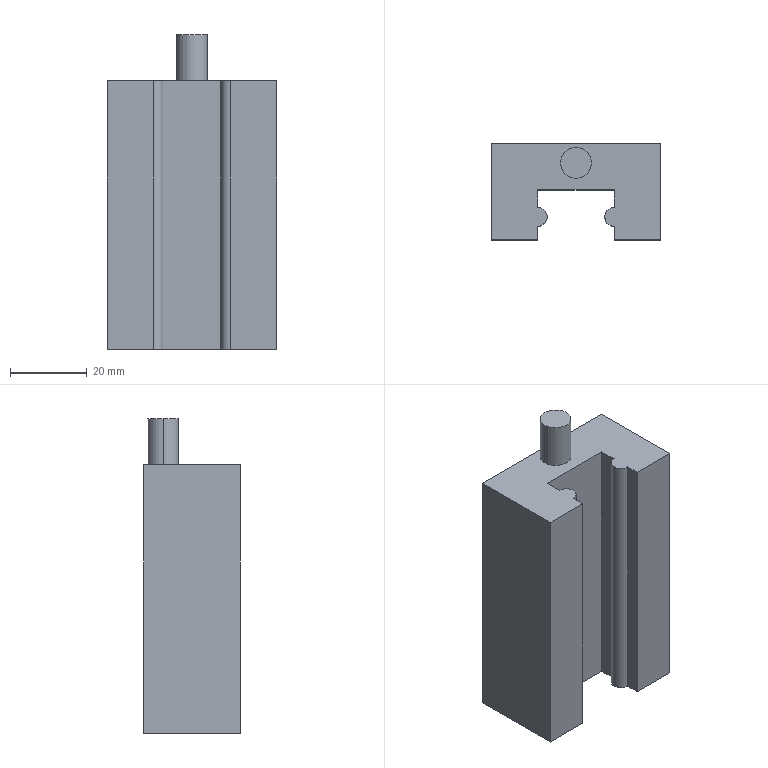Part | SolidWorks | features 3DProfileFeature 1, Extrusion 1, HoleWzd 1, ICE 1 | 1 solid | 34 faces | box 44 x 25 x 81.8 mm | volume 59895 mm3 | cylinder 13 | plane 13 | cone 8 | commonest cylinder face diameters 4.2 x8 5 x3 8 x2
STEP:
#1=CARTESIAN_POINT('',(6.,-12.4,15.9));
#2=VERTEX_POINT('',#1);
#3=CARTESIAN_POINT('',(6.,-12.4,20.1));
#4=VERTEX_POINT('',#3);
#5=CARTESIAN_POINT('',(6.,-12.4,18.));
#6=DIRECTION('',(0.,1.,0.));
#7=DIRECTION('',(0.,0.,1.));
#8=AXIS2_PLACEMENT_3D('',#5,#6,#7);
#9=CIRCLE('',#8,2.1);
#10=EDGE_CURVE('',#2,#4,#9,.T.);
#11=ORIENTED_EDGE('',*,*,#10,.F.);
#12=CARTESIAN_POINT('',(6.,0.,15.9));
#13=VERTEX_POINT('',#12);
#14=CARTESIAN_POINT('',(6.,0.,15.9));
#15=DIRECTION('',(0.,1.,0.));
#16=VECTOR('',#15,1000.);
#17=LINE('',#14,#16);
#18=EDGE_CURVE('',#2,#13,#17,.T.);
#19=ORIENTED_EDGE('',*,*,#18,.T.);
#20=CARTESIAN_POINT('',(6.,0.,20.1));
#21=VERTEX_POINT('',#20);
#22=CARTESIAN_POINT('',(6.,0.,18.));
#23=DIRECTION('',(0.,1.,0.));
#24=DIRECTION('',(0.,0.,1.));
#25=AXIS2_PLACEMENT_3D('',#22,#23,#24);
#26=CIRCLE('',#25,2.1);
#27=EDGE_CURVE('',#13,#21,#26,.T.);
#28=ORIENTED_EDGE('',*,*,#27,.T.);
#29=CARTESIAN_POINT('',(6.,0.,20.1));
#30=DIRECTION('',(0.,1.,0.));
#31=VECTOR('',#30,1000.);
#32=LINE('',#29,#31);
#33=EDGE_CURVE('',#4,#21,#32,.T.);
#34=ORIENTED_EDGE('',*,*,#33,.F.);
#35=EDGE_LOOP('',(#11,#19,#28,#34));
#36=FACE_OUTER_BOUND('',#35,.T.);
#37=CARTESIAN_POINT('',(6.,0.,18.));
#38=DIRECTION('',(0.,1.,0.));
#39=DIRECTION('',(0.,0.,1.));
#40=AXIS2_PLACEMENT_3D('',#37,#38,#39);
#41=CYLINDRICAL_SURFACE('',#40,2.1);
#42=ADVANCED_FACE('',(#36),#41,.F.);
#43=CARTESIAN_POINT('',(6.,-13.662,18.));
#44=VERTEX_POINT('',#43);
#45=CARTESIAN_POINT('',(6.,-12.4,20.1));
#46=DIRECTION('',(0.,0.515,0.8572));
#47=VECTOR('',#46,1000.);
#48=LINE('',#45,#47);
#49=EDGE_CURVE('',#44,#4,#48,.T.);
#50=ORIENTED_EDGE('',*,*,#49,.F.);
#51=CARTESIAN_POINT('',(6.,-12.4,15.9));
#52=DIRECTION('',(0.,0.515,-0.8572));
#53=VECTOR('',#52,1000.);
#54=LINE('',#51,#53);
#55=EDGE_CURVE('',#44,#2,#54,.T.);
#56=ORIENTED_EDGE('',*,*,#55,.T.);
#57=ORIENTED_EDGE('',*,*,#10,.T.);
#58=EDGE_LOOP('',(#50,#56,#57));
#59=FACE_OUTER_BOUND('',#58,.T.);
#60=CARTESIAN_POINT('',(6.,-12.4,18.));
#61=DIRECTION('',(0.,1.,0.));
#62=DIRECTION('',(0.,0.,1.));
#63=AXIS2_PLACEMENT_3D('',#60,#61,#62);
#64=CONICAL_SURFACE('',#63,2.1,1.03);
#65=ADVANCED_FACE('',(#59),#64,.F.);
#66=CARTESIAN_POINT('',(38.,-12.4,15.9));
#67=VERTEX_POINT('',#66);
#68=CARTESIAN_POINT('',(38.,-12.4,20.1));
#69=VERTEX_POINT('',#68);
#70=CARTESIAN_POINT('',(38.,-12.4,18.));
#71=DIRECTION('',(0.,1.,0.));
#72=DIRECTION('',(0.,0.,1.));
#73=AXIS2_PLACEMENT_3D('',#70,#71,#72);
#74=CIRCLE('',#73,2.1);
#75=EDGE_CURVE('',#67,#69,#74,.T.);
#76=ORIENTED_EDGE('',*,*,#75,.F.);
#77=CARTESIAN_POINT('',(38.,0.,15.9));
#78=VERTEX_POINT('',#77);
#79=CARTESIAN_POINT('',(38.,0.,15.9));
#80=DIRECTION('',(0.,1.,0.));
#81=VECTOR('',#80,1000.);
#82=LINE('',#79,#81);
#83=EDGE_CURVE('',#67,#78,#82,.T.);
#84=ORIENTED_EDGE('',*,*,#83,.T.);
#85=CARTESIAN_POINT('',(38.,0.,20.1));
#86=VERTEX_POINT('',#85);
#87=CARTESIAN_POINT('',(38.,0.,18.));
#88=DIRECTION('',(0.,1.,0.));
#89=DIRECTION('',(0.,0.,1.));
#90=AXIS2_PLACEMENT_3D('',#87,#88,#89);
#91=CIRCLE('',#90,2.1);
#92=EDGE_CURVE('',#78,#86,#91,.T.);
#93=ORIENTED_EDGE('',*,*,#92,.T.);
#94=CARTESIAN_POINT('',(38.,0.,20.1));
#95=DIRECTION('',(0.,1.,0.));
#96=VECTOR('',#95,1000.);
#97=LINE('',#94,#96);
#98=EDGE_CURVE('',#69,#86,#97,.T.);
#99=ORIENTED_EDGE('',*,*,#98,.F.);
#100=EDGE_LOOP('',(#76,#84,#93,#99));
#101=FACE_OUTER_BOUND('',#100,.T.);
#102=CARTESIAN_POINT('',(38.,0.,18.));
#103=DIRECTION('',(0.,1.,0.));
#104=DIRECTION('',(0.,0.,1.));
#105=AXIS2_PLACEMENT_3D('',#102,#103,#104);
#106=CYLINDRICAL_SURFACE('',#105,2.1);
#107=ADVANCED_FACE('',(#101),#106,.F.);
#108=CARTESIAN_POINT('',(38.,-13.662,18.));
#109=VERTEX_POINT('',#108);
#110=CARTESIAN_POINT('',(38.,-12.4,20.1));
#111=DIRECTION('',(0.,0.515,0.8572));
#112=VECTOR('',#111,1000.);
#113=LINE('',#110,#112);
#114=EDGE_CURVE('',#109,#69,#113,.T.);
#115=ORIENTED_EDGE('',*,*,#114,.F.);
#116=CARTESIAN_POINT('',(38.,-12.4,15.9));
#117=DIRECTION('',(0.,0.515,-0.8572));
#118=VECTOR('',#117,1000.);
#119=LINE('',#116,#118);
#120=EDGE_CURVE('',#109,#67,#119,.T.);
#121=ORIENTED_EDGE('',*,*,#120,.T.);
#122=ORIENTED_EDGE('',*,*,#75,.T.);
#123=EDGE_LOOP('',(#115,#121,#122));
#124=FACE_OUTER_BOUND('',#123,.T.);
#125=CARTESIAN_POINT('',(38.,-12.4,18.));
#126=DIRECTION('',(0.,1.,0.));
#127=DIRECTION('',(0.,0.,1.));
#128=AXIS2_PLACEMENT_3D('',#125,#126,#127);
#129=CONICAL_SURFACE('',#128,2.1,1.03);
#130=ADVANCED_FACE('',(#124),#129,.F.);
#131=CARTESIAN_POINT('',(6.,-12.4,-20.1));
#132=VERTEX_POINT('',#131);
#133=CARTESIAN_POINT('',(6.,-12.4,-15.9));
#134=VERTEX_POINT('',#133);
#135=CARTESIAN_POINT('',(6.,-12.4,-18.));
#136=DIRECTION('',(0.,1.,0.));
#137=DIRECTION('',(0.,0.,1.));
#138=AXIS2_PLACEMENT_3D('',#135,#136,#137);
#139=CIRCLE('',#138,2.1);
#140=EDGE_CURVE('',#132,#134,#139,.T.);
#141=ORIENTED_EDGE('',*,*,#140,.F.);
#142=CARTESIAN_POINT('',(6.,0.,-20.1));
#143=VERTEX_POINT('',#142);
#144=CARTESIAN_POINT('',(6.,0.,-20.1));
#145=DIRECTION('',(0.,1.,0.));
#146=VECTOR('',#145,1000.);
#147=LINE('',#144,#146);
#148=EDGE_CURVE('',#132,#143,#147,.T.);
#149=ORIENTED_EDGE('',*,*,#148,.T.);
#150=CARTESIAN_POINT('',(6.,0.,-15.9));
#151=VERTEX_POINT('',#150);
#152=CARTESIAN_POINT('',(6.,0.,-18.));
#153=DIRECTION('',(0.,1.,0.));
#154=DIRECTION('',(0.,0.,1.));
#155=AXIS2_PLACEMENT_3D('',#152,#153,#154);
#156=CIRCLE('',#155,2.1);
#157=EDGE_CURVE('',#143,#151,#156,.T.);
#158=ORIENTED_EDGE('',*,*,#157,.T.);
#159=CARTESIAN_POINT('',(6.,0.,-15.9));
#160=DIRECTION('',(0.,1.,0.));
#161=VECTOR('',#160,1000.);
#162=LINE('',#159,#161);
#163=EDGE_CURVE('',#134,#151,#162,.T.);
#164=ORIENTED_EDGE('',*,*,#163,.F.);
#165=EDGE_LOOP('',(#141,#149,#158,#164));
#166=FACE_OUTER_BOUND('',#165,.T.);
#167=CARTESIAN_POINT('',(6.,0.,-18.));
#168=DIRECTION('',(0.,1.,0.));
#169=DIRECTION('',(0.,0.,1.));
#170=AXIS2_PLACEMENT_3D('',#167,#168,#169);
#171=CYLINDRICAL_SURFACE('',#170,2.1);
#172=ADVANCED_FACE('',(#166),#171,.F.);
#173=CARTESIAN_POINT('',(6.,-13.662,-18.));
#174=VERTEX_POINT('',#173);
#175=CARTESIAN_POINT('',(6.,-12.4,-15.9));
#176=DIRECTION('',(0.,0.515,0.8572));
#177=VECTOR('',#176,1000.);
#178=LINE('',#175,#177);
#179=EDGE_CURVE('',#174,#134,#178,.T.);
#180=ORIENTED_EDGE('',*,*,#179,.F.);
#181=CARTESIAN_POINT('',(6.,-12.4,-20.1));
#182=DIRECTION('',(0.,0.515,-0.8572));
#183=VECTOR('',#182,1000.);
#184=LINE('',#181,#183);
#185=EDGE_CURVE('',#174,#132,#184,.T.);
#186=ORIENTED_EDGE('',*,*,#185,.T.);
#187=ORIENTED_EDGE('',*,*,#140,.T.);
#188=EDGE_LOOP('',(#180,#186,#187));
#189=FACE_OUTER_BOUND('',#188,.T.);
#190=CARTESIAN_POINT('',(6.,-12.4,-18.));
#191=DIRECTION('',(0.,1.,0.));
#192=DIRECTION('',(0.,0.,1.));
#193=AXIS2_PLACEMENT_3D('',#190,#191,#192);
#194=CONICAL_SURFACE('',#193,2.1,1.03);
#195=ADVANCED_FACE('',(#189),#194,.F.);
#196=CARTESIAN_POINT('',(38.,-12.4,-20.1));
#197=VERTEX_POINT('',#196);
#198=CARTESIAN_POINT('',(38.,-12.4,-15.9));
#199=VERTEX_POINT('',#198);
#200=CARTESIAN_POINT('',(38.,-12.4,-18.));
#201=DIRECTION('',(0.,1.,0.));
#202=DIRECTION('',(0.,0.,1.));
#203=AXIS2_PLACEMENT_3D('',#200,#201,#202);
#204=CIRCLE('',#203,2.1);
#205=EDGE_CURVE('',#197,#199,#204,.T.);
#206=ORIENTED_EDGE('',*,*,#205,.F.);
#207=CARTESIAN_POINT('',(38.,0.,-20.1));
#208=VERTEX_POINT('',#207);
#209=CARTESIAN_POINT('',(38.,0.,-20.1));
#210=DIRECTION('',(0.,1.,0.));
#211=VECTOR('',#210,1000.);
#212=LINE('',#209,#211);
#213=EDGE_CURVE('',#197,#208,#212,.T.);
#214=ORIENTED_EDGE('',*,*,#213,.T.);
#215=CARTESIAN_POINT('',(38.,0.,-15.9));
#216=VERTEX_POINT('',#215);
#217=CARTESIAN_POINT('',(38.,0.,-18.));
#218=DIRECTION('',(0.,1.,0.));
#219=DIRECTION('',(0.,0.,1.));
#220=AXIS2_PLACEMENT_3D('',#217,#218,#219);
#221=CIRCLE('',#220,2.1);
#222=EDGE_CURVE('',#208,#216,#221,.T.);
#223=ORIENTED_EDGE('',*,*,#222,.T.);
#224=CARTESIAN_POINT('',(38.,0.,-15.9));
#225=DIRECTION('',(0.,1.,0.));
#226=VECTOR('',#225,1000.);
#227=LINE('',#224,#226);
#228=EDGE_CURVE('',#199,#216,#227,.T.);
#229=ORIENTED_EDGE('',*,*,#228,.F.);
#230=EDGE_LOOP('',(#206,#214,#223,#229));
#231=FACE_OUTER_BOUND('',#230,.T.);
#232=CARTESIAN_POINT('',(38.,0.,-18.));
#233=DIRECTION('',(0.,1.,0.));
#234=DIRECTION('',(0.,0.,1.));
#235=AXIS2_PLACEMENT_3D('',#232,#233,#234);
#236=CYLINDRICAL_SURFACE('',#235,2.1);
#237=ADVANCED_FACE('',(#231),#236,.F.);
#238=CARTESIAN_POINT('',(38.,-13.662,-18.));
#239=VERTEX_POINT('',#238);
#240=CARTESIAN_POINT('',(38.,-12.4,-15.9));
#241=DIRECTION('',(0.,0.515,0.8572));
#242=VECTOR('',#241,1000.);
#243=LINE('',#240,#242);
#244=EDGE_CURVE('',#239,#199,#243,.T.);
#245=ORIENTED_EDGE('',*,*,#244,.F.);
#246=CARTESIAN_POINT('',(38.,-12.4,-20.1));
#247=DIRECTION('',(0.,0.515,-0.8572));
#248=VECTOR('',#247,1000.);
#249=LINE('',#246,#248);
#250=EDGE_CURVE('',#239,#197,#249,.T.);
#251=ORIENTED_EDGE('',*,*,#250,.T.);
#252=ORIENTED_EDGE('',*,*,#205,.T.);
#253=EDGE_LOOP('',(#245,#251,#252));
#254=FACE_OUTER_BOUND('',#253,.T.);
#255=CARTESIAN_POINT('',(38.,-12.4,-18.));
#256=DIRECTION('',(0.,1.,0.));
#257=DIRECTION('',(0.,0.,1.));
#258=AXIS2_PLACEMENT_3D('',#255,#256,#257);
#259=CONICAL_SURFACE('',#258,2.1,1.03);
#260=ADVANCED_FACE('',(#254),#259,.F.);
#261=CARTESIAN_POINT('',(26.,-5.,46.9));
#262=VERTEX_POINT('',#261);
#263=CARTESIAN_POINT('',(18.,-5.,46.9));
#264=VERTEX_POINT('',#263);
#265=CARTESIAN_POINT('',(22.,-5.,46.9));
#266=DIRECTION('',(0.,0.,1.));
#267=DIRECTION('',(1.,0.,0.));
#268=AXIS2_PLACEMENT_3D('',#265,#266,#267);
#269=CIRCLE('',#268,4.);
#270=EDGE_CURVE('',#262,#264,#269,.T.);
#271=ORIENTED_EDGE('',*,*,#270,.F.);
#272=CARTESIAN_POINT('',(26.,-5.,34.9));
#273=VERTEX_POINT('',#272);
#274=CARTESIAN_POINT('',(26.,-5.,46.9));
#275=DIRECTION('',(0.,0.,-1.));
#276=VECTOR('',#275,1000.);
#277=LINE('',#274,#276);
#278=EDGE_CURVE('',#262,#273,#277,.T.);
#279=ORIENTED_EDGE('',*,*,#278,.T.);
#280=CARTESIAN_POINT('',(18.,-5.,34.9));
#281=VERTEX_POINT('',#280);
#282=CARTESIAN_POINT('',(22.,-5.,34.9));
#283=DIRECTION('',(0.,0.,1.));
#284=DIRECTION('',(1.,0.,0.));
#285=AXIS2_PLACEMENT_3D('',#282,#283,#284);
#286=CIRCLE('',#285,4.);
#287=EDGE_CURVE('',#273,#281,#286,.T.);
#288=ORIENTED_EDGE('',*,*,#287,.T.);
#289=CARTESIAN_POINT('',(18.,-5.,46.9));
#290=DIRECTION('',(0.,0.,-1.));
#291=VECTOR('',#290,1000.);
#292=LINE('',#289,#291);
#293=EDGE_CURVE('',#264,#281,#292,.T.);
#294=ORIENTED_EDGE('',*,*,#293,.F.);
#295=EDGE_LOOP('',(#271,#279,#288,#294));
#296=FACE_OUTER_BOUND('',#295,.T.);
#297=CARTESIAN_POINT('',(22.,-5.,46.9));
#298=DIRECTION('',(0.,0.,-1.));
#299=DIRECTION('',(-1.,0.,0.));
#300=AXIS2_PLACEMENT_3D('',#297,#298,#299);
#301=CYLINDRICAL_SURFACE('',#300,4.);
#302=ADVANCED_FACE('',(#296),#301,.T.);
#303=CARTESIAN_POINT('',(29.5,-19.,34.9));
#304=VERTEX_POINT('',#303);
#305=CARTESIAN_POINT('',(32.,-21.5,34.9));
#306=VERTEX_POINT('',#305);
#307=CARTESIAN_POINT('',(32.,-19.,34.9));
#308=DIRECTION('',(0.,0.,1.));
#309=DIRECTION('',(1.,0.,0.));
#310=AXIS2_PLACEMENT_3D('',#307,#308,#309);
#311=CIRCLE('',#310,2.5);
#312=EDGE_CURVE('',#304,#306,#311,.T.);
#313=ORIENTED_EDGE('',*,*,#312,.F.);
#314=CARTESIAN_POINT('',(29.5,-19.,-34.9));
#315=VERTEX_POINT('',#314);
#316=CARTESIAN_POINT('',(29.5,-19.,34.9));
#317=DIRECTION('',(0.,0.,-1.));
#318=VECTOR('',#317,1000.);
#319=LINE('',#316,#318);
#320=EDGE_CURVE('',#304,#315,#319,.T.);
#321=ORIENTED_EDGE('',*,*,#320,.T.);
#322=CARTESIAN_POINT('',(32.,-21.5,-34.9));
#323=VERTEX_POINT('',#322);
#324=CARTESIAN_POINT('',(32.,-19.,-34.9));
#325=DIRECTION('',(0.,0.,1.));
#326=DIRECTION('',(1.,0.,0.));
#327=AXIS2_PLACEMENT_3D('',#324,#325,#326);
#328=CIRCLE('',#327,2.5);
#329=EDGE_CURVE('',#315,#323,#328,.T.);
#330=ORIENTED_EDGE('',*,*,#329,.T.);
#331=CARTESIAN_POINT('',(32.,-21.5,34.9));
#332=DIRECTION('',(0.,0.,-1.));
#333=VECTOR('',#332,1000.);
#334=LINE('',#331,#333);
#335=EDGE_CURVE('',#306,#323,#334,.T.);
#336=ORIENTED_EDGE('',*,*,#335,.F.);
#337=EDGE_LOOP('',(#313,#321,#330,#336));
#338=FACE_OUTER_BOUND('',#337,.T.);
#339=CARTESIAN_POINT('',(32.,-19.,34.9));
#340=DIRECTION('',(0.,0.,-1.));
#341=DIRECTION('',(-1.,0.,0.));
#342=AXIS2_PLACEMENT_3D('',#339,#340,#341);
#343=CYLINDRICAL_SURFACE('',#342,2.5);
#344=ADVANCED_FACE('',(#338),#343,.T.);
#345=CARTESIAN_POINT('',(0.,0.,34.9));
#346=VERTEX_POINT('',#345);
#347=CARTESIAN_POINT('',(0.,-25.,34.9));
#348=VERTEX_POINT('',#347);
#349=CARTESIAN_POINT('',(0.,0.,34.9));
#350=DIRECTION('',(0.,-1.,0.));
#351=VECTOR('',#350,1000.);
#352=LINE('',#349,#351);
#353=EDGE_CURVE('',#346,#348,#352,.T.);
#354=ORIENTED_EDGE('',*,*,#353,.T.);
#355=CARTESIAN_POINT('',(12.,-25.,34.9));
#356=VERTEX_POINT('',#355);
#357=CARTESIAN_POINT('',(0.,-25.,34.9));
#358=DIRECTION('',(1.,0.,0.));
#359=VECTOR('',#358,1000.);
#360=LINE('',#357,#359);
#361=EDGE_CURVE('',#348,#356,#360,.T.);
#362=ORIENTED_EDGE('',*,*,#361,.T.);
#363=CARTESIAN_POINT('',(12.,-21.5,34.9));
#364=VERTEX_POINT('',#363);
#365=CARTESIAN_POINT('',(12.,-25.,34.9));
#366=DIRECTION('',(0.,1.,0.));
#367=VECTOR('',#366,1000.);
#368=LINE('',#365,#367);
#369=EDGE_CURVE('',#356,#364,#368,.T.);
#370=ORIENTED_EDGE('',*,*,#369,.T.);
#371=CARTESIAN_POINT('',(12.,-16.5,34.9));
#372=VERTEX_POINT('',#371);
#373=CARTESIAN_POINT('',(12.,-19.,34.9));
#374=DIRECTION('',(0.,0.,1.));
#375=DIRECTION('',(1.,0.,0.));
#376=AXIS2_PLACEMENT_3D('',#373,#374,#375);
#377=CIRCLE('',#376,2.5);
#378=EDGE_CURVE('',#364,#372,#377,.T.);
#379=ORIENTED_EDGE('',*,*,#378,.T.);
#380=CARTESIAN_POINT('',(12.,-12.,34.9));
#381=VERTEX_POINT('',#380);
#382=CARTESIAN_POINT('',(12.,-16.5,34.9));
#383=DIRECTION('',(0.,1.,0.));
#384=VECTOR('',#383,1000.);
#385=LINE('',#382,#384);
#386=EDGE_CURVE('',#372,#381,#385,.T.);
#387=ORIENTED_EDGE('',*,*,#386,.T.);
#388=CARTESIAN_POINT('',(32.,-12.,34.9));
#389=VERTEX_POINT('',#388);
#390=CARTESIAN_POINT('',(12.,-12.,34.9));
#391=DIRECTION('',(1.,0.,0.));
#392=VECTOR('',#391,1000.);
#393=LINE('',#390,#392);
#394=EDGE_CURVE('',#381,#389,#393,.T.);
#395=ORIENTED_EDGE('',*,*,#394,.T.);
#396=CARTESIAN_POINT('',(32.,-16.5,34.9));
#397=VERTEX_POINT('',#396);
#398=CARTESIAN_POINT('',(32.,-16.5,34.9));
#399=DIRECTION('',(0.,-1.,0.));
#400=VECTOR('',#399,1000.);
#401=LINE('',#398,#400);
#402=EDGE_CURVE('',#389,#397,#401,.T.);
#403=ORIENTED_EDGE('',*,*,#402,.T.);
#404=CARTESIAN_POINT('',(32.,-19.,34.9));
#405=DIRECTION('',(0.,0.,1.));
#406=DIRECTION('',(1.,0.,0.));
#407=AXIS2_PLACEMENT_3D('',#404,#405,#406);
#408=CIRCLE('',#407,2.5);
#409=EDGE_CURVE('',#397,#304,#408,.T.);
#410=ORIENTED_EDGE('',*,*,#409,.T.);
#411=ORIENTED_EDGE('',*,*,#312,.T.);
#412=CARTESIAN_POINT('',(32.,-25.,34.9));
#413=VERTEX_POINT('',#412);
#414=CARTESIAN_POINT('',(32.,-25.,34.9));
#415=DIRECTION('',(0.,-1.,0.));
#416=VECTOR('',#415,1000.);
#417=LINE('',#414,#416);
#418=EDGE_CURVE('',#306,#413,#417,.T.);
#419=ORIENTED_EDGE('',*,*,#418,.T.);
#420=CARTESIAN_POINT('',(44.,-25.,34.9));
#421=VERTEX_POINT('',#420);
#422=CARTESIAN_POINT('',(32.,-25.,34.9));
#423=DIRECTION('',(1.,0.,0.));
#424=VECTOR('',#423,1000.);
#425=LINE('',#422,#424);
#426=EDGE_CURVE('',#413,#421,#425,.T.);
#427=ORIENTED_EDGE('',*,*,#426,.T.);
#428=CARTESIAN_POINT('',(44.,0.,34.9));
#429=VERTEX_POINT('',#428);
#430=CARTESIAN_POINT('',(44.,0.,34.9));
#431=DIRECTION('',(0.,1.,0.));
#432=VECTOR('',#431,1000.);
#433=LINE('',#430,#432);
#434=EDGE_CURVE('',#421,#429,#433,.T.);
#435=ORIENTED_EDGE('',*,*,#434,.T.);
#436=CARTESIAN_POINT('',(0.,0.,34.9));
#437=DIRECTION('',(-1.,0.,0.));
#438=VECTOR('',#437,1000.);
#439=LINE('',#436,#438);
#440=EDGE_CURVE('',#429,#346,#439,.T.);
#441=ORIENTED_EDGE('',*,*,#440,.T.);
#442=EDGE_LOOP('',(#354,#362,#370,#379,#387,#395,#403,#410,#411,#419,#427,#435,#441));
#443=FACE_OUTER_BOUND('',#442,.T.);
#444=CARTESIAN_POINT('',(22.,-5.,34.9));
#445=DIRECTION('',(0.,0.,1.));
#446=DIRECTION('',(1.,0.,0.));
#447=AXIS2_PLACEMENT_3D('',#444,#445,#446);
#448=CIRCLE('',#447,4.);
#449=EDGE_CURVE('',#281,#273,#448,.T.);
#450=ORIENTED_EDGE('',*,*,#449,.F.);
#451=ORIENTED_EDGE('',*,*,#287,.F.);
#452=EDGE_LOOP('',(#450,#451));
#453=FACE_BOUND('',#452,.T.);
#454=CARTESIAN_POINT('',(12.,-19.,34.9));
#455=DIRECTION('',(0.,0.,1.));
#456=DIRECTION('',(1.,0.,0.));
#457=AXIS2_PLACEMENT_3D('',#454,#455,#456);
#458=PLANE('',#457);
#459=ADVANCED_FACE('',(#443,#453),#458,.T.);
#460=CARTESIAN_POINT('',(0.,0.,-34.9));
#461=VERTEX_POINT('',#460);
#462=CARTESIAN_POINT('',(0.,-25.,-34.9));
#463=VERTEX_POINT('',#462);
#464=CARTESIAN_POINT('',(0.,0.,-34.9));
#465=DIRECTION('',(0.,-1.,0.));
#466=VECTOR('',#465,1000.);
#467=LINE('',#464,#466);
#468=EDGE_CURVE('',#461,#463,#467,.T.);
#469=ORIENTED_EDGE('',*,*,#468,.T.);
#470=CARTESIAN_POINT('',(0.,-25.,34.9));
#471=DIRECTION('',(0.,0.,-1.));
#472=VECTOR('',#471,1000.);
#473=LINE('',#470,#472);
#474=EDGE_CURVE('',#348,#463,#473,.T.);
#475=ORIENTED_EDGE('',*,*,#474,.F.);
#476=ORIENTED_EDGE('',*,*,#353,.F.);
#477=CARTESIAN_POINT('',(0.,0.,34.9));
#478=DIRECTION('',(0.,0.,-1.));
#479=VECTOR('',#478,1000.);
#480=LINE('',#477,#479);
#481=EDGE_CURVE('',#346,#461,#480,.T.);
#482=ORIENTED_EDGE('',*,*,#481,.T.);
#483=EDGE_LOOP('',(#469,#475,#476,#482));
#484=FACE_OUTER_BOUND('',#483,.T.);
#485=CARTESIAN_POINT('',(0.,0.,34.9));
#486=DIRECTION('',(1.,0.,0.));
#487=DIRECTION('',(0.,1.,0.));
#488=AXIS2_PLACEMENT_3D('',#485,#486,#487);
#489=PLANE('',#488);
#490=ADVANCED_FACE('',(#484),#489,.F.);
#491=CARTESIAN_POINT('',(12.,-25.,-34.9));
#492=VERTEX_POINT('',#491);
#493=CARTESIAN_POINT('',(0.,-25.,-34.9));
#494=DIRECTION('',(1.,0.,0.));
#495=VECTOR('',#494,1000.);
#496=LINE('',#493,#495);
#497=EDGE_CURVE('',#463,#492,#496,.T.);
#498=ORIENTED_EDGE('',*,*,#497,.T.);
#499=CARTESIAN_POINT('',(12.,-25.,34.9));
#500=DIRECTION('',(0.,0.,-1.));
#501=VECTOR('',#500,1000.);
#502=LINE('',#499,#501);
#503=EDGE_CURVE('',#356,#492,#502,.T.);
#504=ORIENTED_EDGE('',*,*,#503,.F.);
#505=ORIENTED_EDGE('',*,*,#361,.F.);
#506=ORIENTED_EDGE('',*,*,#474,.T.);
#507=EDGE_LOOP('',(#498,#504,#505,#506));
#508=FACE_OUTER_BOUND('',#507,.T.);
#509=CARTESIAN_POINT('',(0.,-25.,34.9));
#510=DIRECTION('',(0.,1.,0.));
#511=DIRECTION('',(0.,0.,1.));
#512=AXIS2_PLACEMENT_3D('',#509,#510,#511);
#513=PLANE('',#512);
#514=ADVANCED_FACE('',(#508),#513,.F.);
#515=CARTESIAN_POINT('',(12.,-21.5,-34.9));
#516=VERTEX_POINT('',#515);
#517=CARTESIAN_POINT('',(12.,-25.,-34.9));
#518=DIRECTION('',(0.,1.,0.));
#519=VECTOR('',#518,1000.);
#520=LINE('',#517,#519);
#521=EDGE_CURVE('',#492,#516,#520,.T.);
#522=ORIENTED_EDGE('',*,*,#521,.T.);
#523=CARTESIAN_POINT('',(12.,-21.5,34.9));
#524=DIRECTION('',(0.,0.,-1.));
#525=VECTOR('',#524,1000.);
#526=LINE('',#523,#525);
#527=EDGE_CURVE('',#364,#516,#526,.T.);
#528=ORIENTED_EDGE('',*,*,#527,.F.);
#529=ORIENTED_EDGE('',*,*,#369,.F.);
#530=ORIENTED_EDGE('',*,*,#503,.T.);
#531=EDGE_LOOP('',(#522,#528,#529,#530));
#532=FACE_OUTER_BOUND('',#531,.T.);
#533=CARTESIAN_POINT('',(12.,-25.,34.9));
#534=DIRECTION('',(-1.,0.,0.));
#535=DIRECTION('',(0.,0.,1.));
#536=AXIS2_PLACEMENT_3D('',#533,#534,#535);
#537=PLANE('',#536);
#538=ADVANCED_FACE('',(#532),#537,.F.);
#539=CARTESIAN_POINT('',(12.,-16.5,-34.9));
#540=VERTEX_POINT('',#539);
#541=CARTESIAN_POINT('',(12.,-19.,-34.9));
#542=DIRECTION('',(0.,0.,1.));
#543=DIRECTION('',(1.,0.,0.));
#544=AXIS2_PLACEMENT_3D('',#541,#542,#543);
#545=CIRCLE('',#544,2.5);
#546=EDGE_CURVE('',#516,#540,#545,.T.);
#547=ORIENTED_EDGE('',*,*,#546,.T.);
#548=CARTESIAN_POINT('',(12.,-16.5,34.9));
#549=DIRECTION('',(0.,0.,-1.));
#550=VECTOR('',#549,1000.);
#551=LINE('',#548,#550);
#552=EDGE_CURVE('',#372,#540,#551,.T.);
#553=ORIENTED_EDGE('',*,*,#552,.F.);
#554=ORIENTED_EDGE('',*,*,#378,.F.);
#555=ORIENTED_EDGE('',*,*,#527,.T.);
#556=EDGE_LOOP('',(#547,#553,#554,#555));
#557=FACE_OUTER_BOUND('',#556,.T.);
#558=CARTESIAN_POINT('',(12.,-19.,34.9));
#559=DIRECTION('',(0.,0.,-1.));
#560=DIRECTION('',(-1.,0.,0.));
#561=AXIS2_PLACEMENT_3D('',#558,#559,#560);
#562=CYLINDRICAL_SURFACE('',#561,2.5);
#563=ADVANCED_FACE('',(#557),#562,.T.);
#564=CARTESIAN_POINT('',(12.,-12.,-34.9));
#565=VERTEX_POINT('',#564);
#566=CARTESIAN_POINT('',(12.,-16.5,-34.9));
#567=DIRECTION('',(0.,1.,0.));
#568=VECTOR('',#567,1000.);
#569=LINE('',#566,#568);
#570=EDGE_CURVE('',#540,#565,#569,.T.);
#571=ORIENTED_EDGE('',*,*,#570,.T.);
#572=CARTESIAN_POINT('',(12.,-12.,34.9));
#573=DIRECTION('',(0.,0.,-1.));
#574=VECTOR('',#573,1000.);
#575=LINE('',#572,#574);
#576=EDGE_CURVE('',#381,#565,#575,.T.);
#577=ORIENTED_EDGE('',*,*,#576,.F.);
#578=ORIENTED_EDGE('',*,*,#386,.F.);
#579=ORIENTED_EDGE('',*,*,#552,.T.);
#580=EDGE_LOOP('',(#571,#577,#578,#579));
#581=FACE_OUTER_BOUND('',#580,.T.);
#582=CARTESIAN_POINT('',(12.,-16.5,34.9));
#583=DIRECTION('',(-1.,0.,0.));
#584=DIRECTION('',(0.,0.,1.));
#585=AXIS2_PLACEMENT_3D('',#582,#583,#584);
#586=PLANE('',#585);
#587=ADVANCED_FACE('',(#581),#586,.F.);
#588=CARTESIAN_POINT('',(32.,-12.,-34.9));
#589=VERTEX_POINT('',#588);
#590=CARTESIAN_POINT('',(12.,-12.,-34.9));
#591=DIRECTION('',(1.,0.,0.));
#592=VECTOR('',#591,1000.);
#593=LINE('',#590,#592);
#594=EDGE_CURVE('',#565,#589,#593,.T.);
#595=ORIENTED_EDGE('',*,*,#594,.T.);
#596=CARTESIAN_POINT('',(32.,-12.,34.9));
#597=DIRECTION('',(0.,0.,-1.));
#598=VECTOR('',#597,1000.);
#599=LINE('',#596,#598);
#600=EDGE_CURVE('',#389,#589,#599,.T.);
#601=ORIENTED_EDGE('',*,*,#600,.F.);
#602=ORIENTED_EDGE('',*,*,#394,.F.);
#603=ORIENTED_EDGE('',*,*,#576,.T.);
#604=EDGE_LOOP('',(#595,#601,#602,#603));
#605=FACE_OUTER_BOUND('',#604,.T.);
#606=CARTESIAN_POINT('',(12.,-12.,34.9));
#607=DIRECTION('',(0.,1.,0.));
#608=DIRECTION('',(0.,0.,1.));
#609=AXIS2_PLACEMENT_3D('',#606,#607,#608);
#610=PLANE('',#609);
#611=ADVANCED_FACE('',(#605),#610,.F.);
#612=CARTESIAN_POINT('',(32.,-16.5,-34.9));
#613=VERTEX_POINT('',#612);
#614=CARTESIAN_POINT('',(32.,-16.5,-34.9));
#615=DIRECTION('',(0.,-1.,0.));
#616=VECTOR('',#615,1000.);
#617=LINE('',#614,#616);
#618=EDGE_CURVE('',#589,#613,#617,.T.);
#619=ORIENTED_EDGE('',*,*,#618,.T.);
#620=CARTESIAN_POINT('',(32.,-16.5,34.9));
#621=DIRECTION('',(0.,0.,-1.));
#622=VECTOR('',#621,1000.);
#623=LINE('',#620,#622);
#624=EDGE_CURVE('',#397,#613,#623,.T.);
#625=ORIENTED_EDGE('',*,*,#624,.F.);
#626=ORIENTED_EDGE('',*,*,#402,.F.);
#627=ORIENTED_EDGE('',*,*,#600,.T.);
#628=EDGE_LOOP('',(#619,#625,#626,#627));
#629=FACE_OUTER_BOUND('',#628,.T.);
#630=CARTESIAN_POINT('',(32.,-16.5,34.9));
#631=DIRECTION('',(1.,0.,0.));
#632=DIRECTION('',(0.,0.,-1.));
#633=AXIS2_PLACEMENT_3D('',#630,#631,#632);
#634=PLANE('',#633);
#635=ADVANCED_FACE('',(#629),#634,.F.);
#636=ORIENTED_EDGE('',*,*,#320,.F.);
#637=ORIENTED_EDGE('',*,*,#409,.F.);
#638=ORIENTED_EDGE('',*,*,#624,.T.);
#639=CARTESIAN_POINT('',(32.,-19.,-34.9));
#640=DIRECTION('',(0.,0.,1.));
#641=DIRECTION('',(1.,0.,0.));
#642=AXIS2_PLACEMENT_3D('',#639,#640,#641);
#643=CIRCLE('',#642,2.5);
#644=EDGE_CURVE('',#613,#315,#643,.T.);
#645=ORIENTED_EDGE('',*,*,#644,.T.);
#646=EDGE_LOOP('',(#636,#637,#638,#645));
#647=FACE_OUTER_BOUND('',#646,.T.);
#648=CARTESIAN_POINT('',(32.,-19.,34.9));
#649=DIRECTION('',(0.,0.,-1.));
#650=DIRECTION('',(-1.,0.,0.));
#651=AXIS2_PLACEMENT_3D('',#648,#649,#650);
#652=CYLINDRICAL_SURFACE('',#651,2.5);
#653=ADVANCED_FACE('',(#647),#652,.T.);
#654=CARTESIAN_POINT('',(32.,-25.,-34.9));
#655=VERTEX_POINT('',#654);
#656=CARTESIAN_POINT('',(32.,-25.,-34.9));
#657=DIRECTION('',(0.,-1.,0.));
#658=VECTOR('',#657,1000.);
#659=LINE('',#656,#658);
#660=EDGE_CURVE('',#323,#655,#659,.T.);
#661=ORIENTED_EDGE('',*,*,#660,.T.);
#662=CARTESIAN_POINT('',(32.,-25.,34.9));
#663=DIRECTION('',(0.,0.,-1.));
#664=VECTOR('',#663,1000.);
#665=LINE('',#662,#664);
#666=EDGE_CURVE('',#413,#655,#665,.T.);
#667=ORIENTED_EDGE('',*,*,#666,.F.);
#668=ORIENTED_EDGE('',*,*,#418,.F.);
#669=ORIENTED_EDGE('',*,*,#335,.T.);
#670=EDGE_LOOP('',(#661,#667,#668,#669));
#671=FACE_OUTER_BOUND('',#670,.T.);
#672=CARTESIAN_POINT('',(32.,-25.,34.9));
#673=DIRECTION('',(1.,0.,0.));
#674=DIRECTION('',(0.,0.,-1.));
#675=AXIS2_PLACEMENT_3D('',#672,#673,#674);
#676=PLANE('',#675);
#677=ADVANCED_FACE('',(#671),#676,.F.);
#678=CARTESIAN_POINT('',(44.,-25.,-34.9));
#679=VERTEX_POINT('',#678);
#680=CARTESIAN_POINT('',(32.,-25.,-34.9));
#681=DIRECTION('',(1.,0.,0.));
#682=VECTOR('',#681,1000.);
#683=LINE('',#680,#682);
#684=EDGE_CURVE('',#655,#679,#683,.T.);
#685=ORIENTED_EDGE('',*,*,#684,.T.);
#686=CARTESIAN_POINT('',(44.,-25.,34.9));
#687=DIRECTION('',(0.,0.,-1.));
#688=VECTOR('',#687,1000.);
#689=LINE('',#686,#688);
#690=EDGE_CURVE('',#421,#679,#689,.T.);
#691=ORIENTED_EDGE('',*,*,#690,.F.);
#692=ORIENTED_EDGE('',*,*,#426,.F.);
#693=ORIENTED_EDGE('',*,*,#666,.T.);
#694=EDGE_LOOP('',(#685,#691,#692,#693));
#695=FACE_OUTER_BOUND('',#694,.T.);
#696=CARTESIAN_POINT('',(32.,-25.,34.9));
#697=DIRECTION('',(0.,1.,0.));
#698=DIRECTION('',(0.,0.,1.));
#699=AXIS2_PLACEMENT_3D('',#696,#697,#698);
#700=PLANE('',#699);
#701=ADVANCED_FACE('',(#695),#700,.F.);
#702=CARTESIAN_POINT('',(44.,0.,-34.9));
#703=VERTEX_POINT('',#702);
#704=CARTESIAN_POINT('',(44.,0.,-34.9));
#705=DIRECTION('',(0.,1.,0.));
#706=VECTOR('',#705,1000.);
#707=LINE('',#704,#706);
#708=EDGE_CURVE('',#679,#703,#707,.T.);
#709=ORIENTED_EDGE('',*,*,#708,.T.);
#710=CARTESIAN_POINT('',(44.,0.,34.9));
#711=DIRECTION('',(0.,0.,-1.));
#712=VECTOR('',#711,1000.);
#713=LINE('',#710,#712);
#714=EDGE_CURVE('',#429,#703,#713,.T.);
#715=ORIENTED_EDGE('',*,*,#714,.F.);
#716=ORIENTED_EDGE('',*,*,#434,.F.);
#717=ORIENTED_EDGE('',*,*,#690,.T.);
#718=EDGE_LOOP('',(#709,#715,#716,#717));
#719=FACE_OUTER_BOUND('',#718,.T.);
#720=CARTESIAN_POINT('',(44.,0.,34.9));
#721=DIRECTION('',(-1.,0.,0.));
#722=DIRECTION('',(0.,0.,1.));
#723=AXIS2_PLACEMENT_3D('',#720,#721,#722);
#724=PLANE('',#723);
#725=ADVANCED_FACE('',(#719),#724,.F.);
#726=CARTESIAN_POINT('',(6.,0.,18.));
#727=DIRECTION('',(0.,1.,0.));
#728=DIRECTION('',(0.,0.,1.));
#729=AXIS2_PLACEMENT_3D('',#726,#727,#728);
#730=CIRCLE('',#729,2.1);
#731=EDGE_CURVE('',#21,#13,#730,.T.);
#732=ORIENTED_EDGE('',*,*,#731,.F.);
#733=ORIENTED_EDGE('',*,*,#27,.F.);
#734=EDGE_LOOP('',(#732,#733));
#735=FACE_BOUND('',#734,.T.);
#736=CARTESIAN_POINT('',(38.,0.,18.));
#737=DIRECTION('',(0.,1.,0.));
#738=DIRECTION('',(0.,0.,1.));
#739=AXIS2_PLACEMENT_3D('',#736,#737,#738);
#740=CIRCLE('',#739,2.1);
#741=EDGE_CURVE('',#86,#78,#740,.T.);
#742=ORIENTED_EDGE('',*,*,#741,.F.);
#743=ORIENTED_EDGE('',*,*,#92,.F.);
#744=EDGE_LOOP('',(#742,#743));
#745=FACE_BOUND('',#744,.T.);
#746=CARTESIAN_POINT('',(6.,0.,-18.));
#747=DIRECTION('',(0.,1.,0.));
#748=DIRECTION('',(0.,0.,1.));
#749=AXIS2_PLACEMENT_3D('',#746,#747,#748);
#750=CIRCLE('',#749,2.1);
#751=EDGE_CURVE('',#151,#143,#750,.T.);
#752=ORIENTED_EDGE('',*,*,#751,.F.);
#753=ORIENTED_EDGE('',*,*,#157,.F.);
#754=EDGE_LOOP('',(#752,#753));
#755=FACE_BOUND('',#754,.T.);
#756=CARTESIAN_POINT('',(38.,0.,-18.));
#757=DIRECTION('',(0.,1.,0.));
#758=DIRECTION('',(0.,0.,1.));
#759=AXIS2_PLACEMENT_3D('',#756,#757,#758);
#760=CIRCLE('',#759,2.1);
#761=EDGE_CURVE('',#216,#208,#760,.T.);
#762=ORIENTED_EDGE('',*,*,#761,.F.);
#763=ORIENTED_EDGE('',*,*,#222,.F.);
#764=EDGE_LOOP('',(#762,#763));
#765=FACE_BOUND('',#764,.T.);
#766=CARTESIAN_POINT('',(0.,0.,-34.9));
#767=DIRECTION('',(-1.,0.,0.));
#768=VECTOR('',#767,1000.);
#769=LINE('',#766,#768);
#770=EDGE_CURVE('',#703,#461,#769,.T.);
#771=ORIENTED_EDGE('',*,*,#770,.T.);
#772=ORIENTED_EDGE('',*,*,#481,.F.);
#773=ORIENTED_EDGE('',*,*,#440,.F.);
#774=ORIENTED_EDGE('',*,*,#714,.T.);
#775=EDGE_LOOP('',(#771,#772,#773,#774));
#776=FACE_OUTER_BOUND('',#775,.T.);
#777=CARTESIAN_POINT('',(0.,0.,34.9));
#778=DIRECTION('',(0.,-1.,0.));
#779=DIRECTION('',(0.,0.,-1.));
#780=AXIS2_PLACEMENT_3D('',#777,#778,#779);
#781=PLANE('',#780);
#782=ADVANCED_FACE('',(#735,#745,#755,#765,#776),#781,.F.);
#783=ORIENTED_EDGE('',*,*,#468,.F.);
#784=ORIENTED_EDGE('',*,*,#770,.F.);
#785=ORIENTED_EDGE('',*,*,#708,.F.);
#786=ORIENTED_EDGE('',*,*,#684,.F.);
#787=ORIENTED_EDGE('',*,*,#660,.F.);
#788=ORIENTED_EDGE('',*,*,#329,.F.);
#789=ORIENTED_EDGE('',*,*,#644,.F.);
#790=ORIENTED_EDGE('',*,*,#618,.F.);
#791=ORIENTED_EDGE('',*,*,#594,.F.);
#792=ORIENTED_EDGE('',*,*,#570,.F.);
#793=ORIENTED_EDGE('',*,*,#546,.F.);
#794=ORIENTED_EDGE('',*,*,#521,.F.);
#795=ORIENTED_EDGE('',*,*,#497,.F.);
#796=EDGE_LOOP('',(#783,#784,#785,#786,#787,#788,#789,#790,#791,#792,#793,#794,#795));
#797=FACE_OUTER_BOUND('',#796,.T.);
#798=CARTESIAN_POINT('',(12.,-19.,-34.9));
#799=DIRECTION('',(0.,0.,1.));
#800=DIRECTION('',(1.,0.,0.));
#801=AXIS2_PLACEMENT_3D('',#798,#799,#800);
#802=PLANE('',#801);
#803=ADVANCED_FACE('',(#797),#802,.F.);
#804=ORIENTED_EDGE('',*,*,#278,.F.);
#805=CARTESIAN_POINT('',(22.,-5.,46.9));
#806=DIRECTION('',(0.,0.,1.));
#807=DIRECTION('',(1.,0.,0.));
#808=AXIS2_PLACEMENT_3D('',#805,#806,#807);
#809=CIRCLE('',#808,4.);
#810=EDGE_CURVE('',#264,#262,#809,.T.);
#811=ORIENTED_EDGE('',*,*,#810,.F.);
#812=ORIENTED_EDGE('',*,*,#293,.T.);
#813=ORIENTED_EDGE('',*,*,#449,.T.);
#814=EDGE_LOOP('',(#804,#811,#812,#813));
#815=FACE_OUTER_BOUND('',#814,.T.);
#816=CARTESIAN_POINT('',(22.,-5.,46.9));
#817=DIRECTION('',(0.,0.,-1.));
#818=DIRECTION('',(-1.,0.,0.));
#819=AXIS2_PLACEMENT_3D('',#816,#817,#818);
#820=CYLINDRICAL_SURFACE('',#819,4.);
#821=ADVANCED_FACE('',(#815),#820,.T.);
#822=ORIENTED_EDGE('',*,*,#810,.T.);
#823=ORIENTED_EDGE('',*,*,#270,.T.);
#824=EDGE_LOOP('',(#822,#823));
#825=FACE_OUTER_BOUND('',#824,.T.);
#826=CARTESIAN_POINT('',(22.,-5.,46.9));
#827=DIRECTION('',(0.,0.,1.));
#828=DIRECTION('',(1.,0.,0.));
#829=AXIS2_PLACEMENT_3D('',#826,#827,#828);
#830=PLANE('',#829);
#831=ADVANCED_FACE('',(#825),#830,.T.);
#832=ORIENTED_EDGE('',*,*,#250,.F.);
#833=ORIENTED_EDGE('',*,*,#244,.T.);
#834=CARTESIAN_POINT('',(38.,-12.4,-18.));
#835=DIRECTION('',(0.,1.,0.));
#836=DIRECTION('',(0.,0.,1.));
#837=AXIS2_PLACEMENT_3D('',#834,#835,#836);
#838=CIRCLE('',#837,2.1);
#839=EDGE_CURVE('',#199,#197,#838,.T.);
#840=ORIENTED_EDGE('',*,*,#839,.T.);
#841=EDGE_LOOP('',(#832,#833,#840));
#842=FACE_OUTER_BOUND('',#841,.T.);
#843=CARTESIAN_POINT('',(38.,-12.4,-18.));
#844=DIRECTION('',(0.,1.,0.));
#845=DIRECTION('',(0.,0.,1.));
#846=AXIS2_PLACEMENT_3D('',#843,#844,#845);
#847=CONICAL_SURFACE('',#846,2.1,1.03);
#848=ADVANCED_FACE('',(#842),#847,.F.);
#849=ORIENTED_EDGE('',*,*,#213,.F.);
#850=ORIENTED_EDGE('',*,*,#839,.F.);
#851=ORIENTED_EDGE('',*,*,#228,.T.);
#852=ORIENTED_EDGE('',*,*,#761,.T.);
#853=EDGE_LOOP('',(#849,#850,#851,#852));
#854=FACE_OUTER_BOUND('',#853,.T.);
#855=CARTESIAN_POINT('',(38.,0.,-18.));
#856=DIRECTION('',(0.,1.,0.));
#857=DIRECTION('',(0.,0.,1.));
#858=AXIS2_PLACEMENT_3D('',#855,#856,#857);
#859=CYLINDRICAL_SURFACE('',#858,2.1);
#860=ADVANCED_FACE('',(#854),#859,.F.);
#861=ORIENTED_EDGE('',*,*,#185,.F.);
#862=ORIENTED_EDGE('',*,*,#179,.T.);
#863=CARTESIAN_POINT('',(6.,-12.4,-18.));
#864=DIRECTION('',(0.,1.,0.));
#865=DIRECTION('',(0.,0.,1.));
#866=AXIS2_PLACEMENT_3D('',#863,#864,#865);
#867=CIRCLE('',#866,2.1);
#868=EDGE_CURVE('',#134,#132,#867,.T.);
#869=ORIENTED_EDGE('',*,*,#868,.T.);
#870=EDGE_LOOP('',(#861,#862,#869));
#871=FACE_OUTER_BOUND('',#870,.T.);
#872=CARTESIAN_POINT('',(6.,-12.4,-18.));
#873=DIRECTION('',(0.,1.,0.));
#874=DIRECTION('',(0.,0.,1.));
#875=AXIS2_PLACEMENT_3D('',#872,#873,#874);
#876=CONICAL_SURFACE('',#875,2.1,1.03);
#877=ADVANCED_FACE('',(#871),#876,.F.);
#878=ORIENTED_EDGE('',*,*,#148,.F.);
#879=ORIENTED_EDGE('',*,*,#868,.F.);
#880=ORIENTED_EDGE('',*,*,#163,.T.);
#881=ORIENTED_EDGE('',*,*,#751,.T.);
#882=EDGE_LOOP('',(#878,#879,#880,#881));
#883=FACE_OUTER_BOUND('',#882,.T.);
#884=CARTESIAN_POINT('',(6.,0.,-18.));
#885=DIRECTION('',(0.,1.,0.));
#886=DIRECTION('',(0.,0.,1.));
#887=AXIS2_PLACEMENT_3D('',#884,#885,#886);
#888=CYLINDRICAL_SURFACE('',#887,2.1);
#889=ADVANCED_FACE('',(#883),#888,.F.);
#890=ORIENTED_EDGE('',*,*,#120,.F.);
#891=ORIENTED_EDGE('',*,*,#114,.T.);
#892=CARTESIAN_POINT('',(38.,-12.4,18.));
#893=DIRECTION('',(0.,1.,0.));
#894=DIRECTION('',(0.,0.,1.));
#895=AXIS2_PLACEMENT_3D('',#892,#893,#894);
#896=CIRCLE('',#895,2.1);
#897=EDGE_CURVE('',#69,#67,#896,.T.);
#898=ORIENTED_EDGE('',*,*,#897,.T.);
#899=EDGE_LOOP('',(#890,#891,#898));
#900=FACE_OUTER_BOUND('',#899,.T.);
#901=CARTESIAN_POINT('',(38.,-12.4,18.));
#902=DIRECTION('',(0.,1.,0.));
#903=DIRECTION('',(0.,0.,1.));
#904=AXIS2_PLACEMENT_3D('',#901,#902,#903);
#905=CONICAL_SURFACE('',#904,2.1,1.03);
#906=ADVANCED_FACE('',(#900),#905,.F.);
#907=ORIENTED_EDGE('',*,*,#83,.F.);
#908=ORIENTED_EDGE('',*,*,#897,.F.);
#909=ORIENTED_EDGE('',*,*,#98,.T.);
#910=ORIENTED_EDGE('',*,*,#741,.T.);
#911=EDGE_LOOP('',(#907,#908,#909,#910));
#912=FACE_OUTER_BOUND('',#911,.T.);
#913=CARTESIAN_POINT('',(38.,0.,18.));
#914=DIRECTION('',(0.,1.,0.));
#915=DIRECTION('',(0.,0.,1.));
#916=AXIS2_PLACEMENT_3D('',#913,#914,#915);
#917=CYLINDRICAL_SURFACE('',#916,2.1);
#918=ADVANCED_FACE('',(#912),#917,.F.);
#919=ORIENTED_EDGE('',*,*,#55,.F.);
#920=ORIENTED_EDGE('',*,*,#49,.T.);
#921=CARTESIAN_POINT('',(6.,-12.4,18.));
#922=DIRECTION('',(0.,1.,0.));
#923=DIRECTION('',(0.,0.,1.));
#924=AXIS2_PLACEMENT_3D('',#921,#922,#923);
#925=CIRCLE('',#924,2.1);
#926=EDGE_CURVE('',#4,#2,#925,.T.);
#927=ORIENTED_EDGE('',*,*,#926,.T.);
#928=EDGE_LOOP('',(#919,#920,#927));
#929=FACE_OUTER_BOUND('',#928,.T.);
#930=CARTESIAN_POINT('',(6.,-12.4,18.));
#931=DIRECTION('',(0.,1.,0.));
#932=DIRECTION('',(0.,0.,1.));
#933=AXIS2_PLACEMENT_3D('',#930,#931,#932);
#934=CONICAL_SURFACE('',#933,2.1,1.03);
#935=ADVANCED_FACE('',(#929),#934,.F.);
#936=ORIENTED_EDGE('',*,*,#18,.F.);
#937=ORIENTED_EDGE('',*,*,#926,.F.);
#938=ORIENTED_EDGE('',*,*,#33,.T.);
#939=ORIENTED_EDGE('',*,*,#731,.T.);
#940=EDGE_LOOP('',(#936,#937,#938,#939));
#941=FACE_OUTER_BOUND('',#940,.T.);
#942=CARTESIAN_POINT('',(6.,0.,18.));
#943=DIRECTION('',(0.,1.,0.));
#944=DIRECTION('',(0.,0.,1.));
#945=AXIS2_PLACEMENT_3D('',#942,#943,#944);
#946=CYLINDRICAL_SURFACE('',#945,2.1);
#947=ADVANCED_FACE('',(#941),#946,.F.);
#948=CLOSED_SHELL('',(#42,#65,#107,#130,#172,#195,#237,#260,#302,#344,#459,#490,#514,#538,#563,#587,#611,#635,#653,#677,#701,#725,#782,#803,#821,#831,#848,#860,#877,#889,#906,#918,#935,#947));
#949=MANIFOLD_SOLID_BREP('',#948);
#950=CARTESIAN_POINT('',(0.,0.,0.));
#951=DIRECTION('',(0.,0.,1.));
#952=DIRECTION('',(1.,0.,0.));
#953=AXIS2_PLACEMENT_3D('',#950,#951,#952);
#954=(LENGTH_UNIT()NAMED_UNIT(*)SI_UNIT(.MILLI.,.METRE.));
#955=UNCERTAINTY_MEASURE_WITH_UNIT(LENGTH_MEASURE(0.00001),#954,'','');
#956=(NAMED_UNIT(*)PLANE_ANGLE_UNIT()SI_UNIT($,.RADIAN.));
#957=(NAMED_UNIT(*)SI_UNIT($,.STERADIAN.)SOLID_ANGLE_UNIT());
#958=(GEOMETRIC_REPRESENTATION_CONTEXT(3)GLOBAL_UNCERTAINTY_ASSIGNED_CONTEXT((#955))GLOBAL_UNIT_ASSIGNED_CONTEXT((#954,#956,#957))REPRESENTATION_CONTEXT('',''));
#959=ADVANCED_BREP_SHAPE_REPRESENTATION('',(#949,#953),#958);